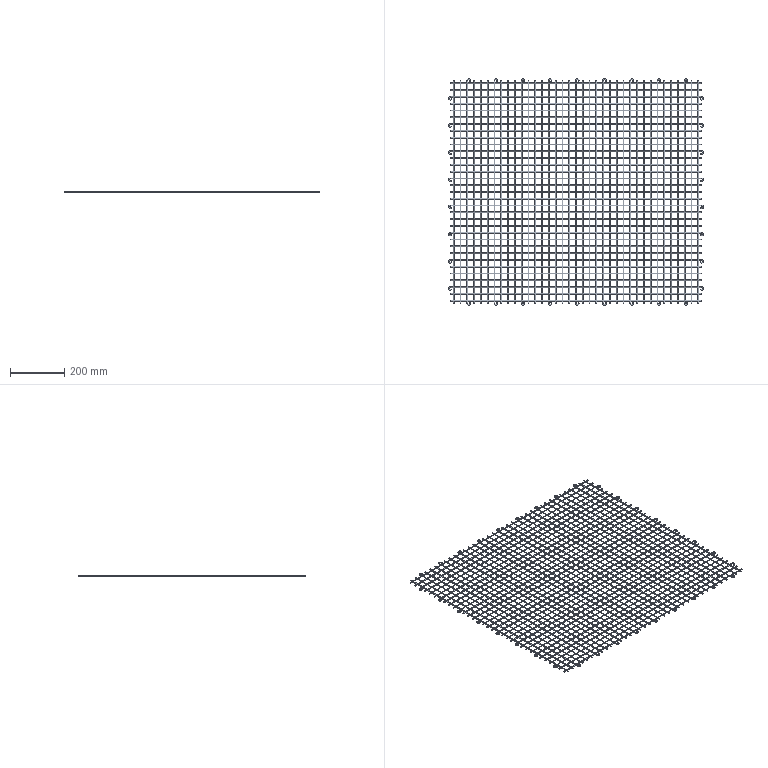Part | STEP file | 750078470 | 104 solids | 468 faces | box 938 x 833 x 3 mm | volume 434942 mm3 | plane 208 | cylinder 140 | spline 120 | commonest cylinder face diameters 3 x140